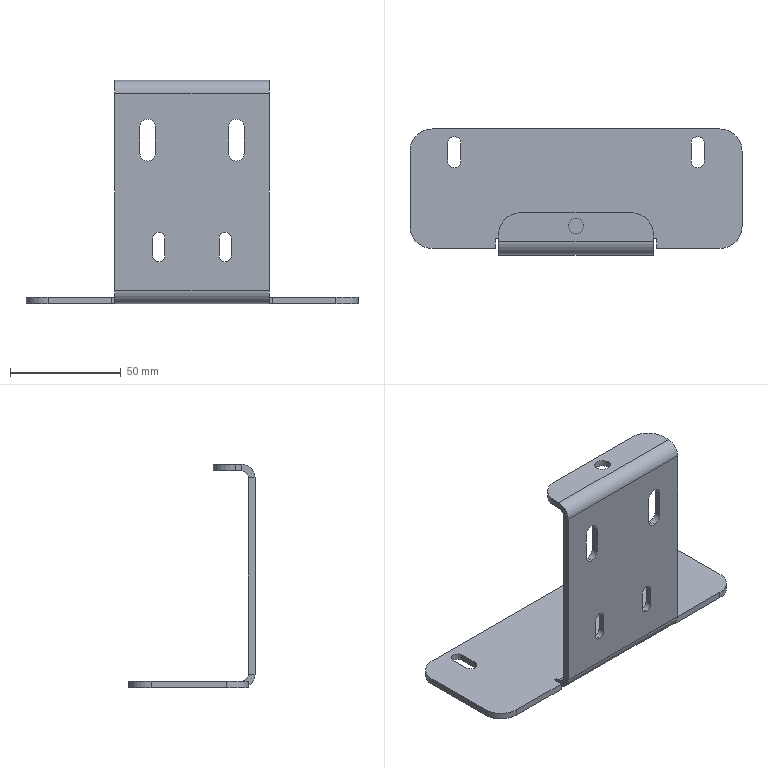Part | NX | features BREP 1 | 1 solid | 66 faces | box 150 x 57 x 101 mm | volume 45917 mm3 | plane 38 | cylinder 28 | commonest cylinder face diameters 7 x8 5.5 x6 6 x6 20 x6 12 x2